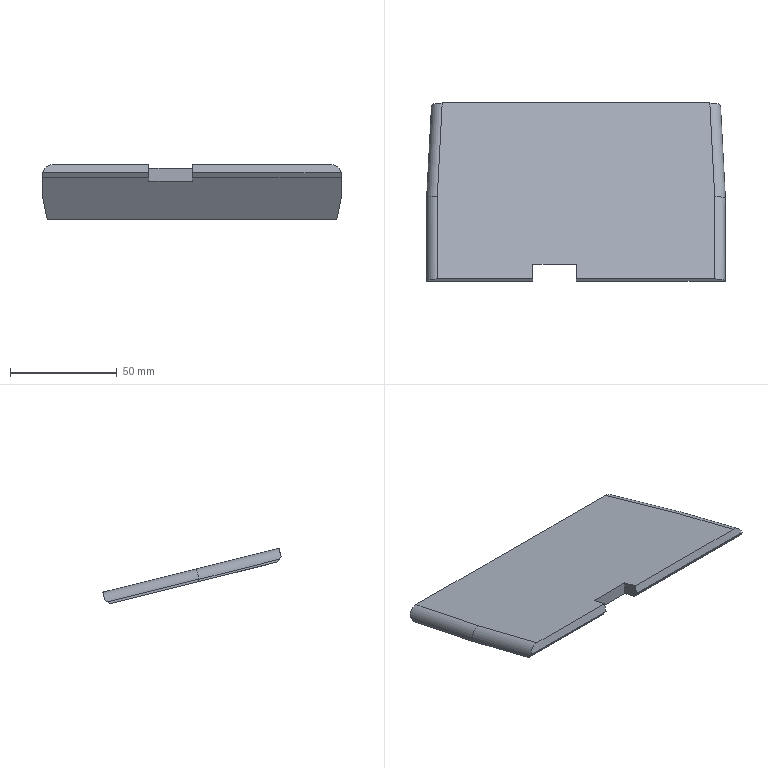Part | STEP file | WEAR-PLATE2_id674_x_t | 1 solid | 19 faces | box 140 x 83.443 x 25.901 mm | volume 68382 mm3 | plane 15 | cylinder 4 | commonest cylinder face diameters 10 x4
STEP:
#1=CARTESIAN_POINT('',(45.,1.133,224.747));
#2=VERTEX_POINT('',#1);
#3=CARTESIAN_POINT('',(50.,0.06233,219.926));
#4=VERTEX_POINT('',#3);
#5=CARTESIAN_POINT('',(45.,-0.07625,219.896));
#6=DIRECTION('',(-0.0254,0.97,-0.2418));
#7=DIRECTION('',(-0.9997,-0.02465,0.006145));
#8=AXIS2_PLACEMENT_3D('',#5,#6,#7);
#9=ELLIPSE('',#8,5.002,5.);
#10=EDGE_CURVE('',#2,#4,#9,.T.);
#11=ORIENTED_EDGE('',*,*,#10,.F.);
#12=CARTESIAN_POINT('',(45.,-37.475,234.373));
#13=VERTEX_POINT('',#12);
#14=CARTESIAN_POINT('',(45.,-37.475,234.373));
#15=DIRECTION('',(0.,0.9703,-0.2419));
#16=VECTOR('',#15,1.);
#17=LINE('',#14,#16);
#18=EDGE_CURVE('',#13,#2,#17,.T.);
#19=ORIENTED_EDGE('',*,*,#18,.F.);
#20=CARTESIAN_POINT('',(49.899,-38.443,230.492));
#21=VERTEX_POINT('',#20);
#22=CARTESIAN_POINT('',(45.,-38.685,229.522));
#23=DIRECTION('',(0.,-0.9703,0.2419));
#24=DIRECTION('',(0.,-0.2419,-0.9703));
#25=AXIS2_PLACEMENT_3D('',#22,#23,#24);
#26=CIRCLE('',#25,5.);
#27=EDGE_CURVE('',#21,#13,#26,.T.);
#28=ORIENTED_EDGE('',*,*,#27,.F.);
#29=CARTESIAN_POINT('',(50.,-37.714,229.28));
#30=VERTEX_POINT('',#29);
#31=CARTESIAN_POINT('',(45.,-37.714,229.28));
#32=DIRECTION('',(0.,0.8572,0.515));
#33=DIRECTION('',(0.,-0.515,0.8572));
#34=AXIS2_PLACEMENT_3D('',#31,#32,#33);
#35=ELLIPSE('',#34,7.071,5.);
#36=EDGE_CURVE('',#21,#30,#35,.T.);
#37=ORIENTED_EDGE('',*,*,#36,.T.);
#38=CARTESIAN_POINT('',(50.,0.05468,219.863));
#39=VERTEX_POINT('',#38);
#40=CARTESIAN_POINT('',(50.,-37.714,229.28));
#41=DIRECTION('',(0.,0.9703,-0.2419));
#42=VECTOR('',#41,1.);
#43=LINE('',#40,#42);
#44=EDGE_CURVE('',#30,#39,#43,.T.);
#45=ORIENTED_EDGE('',*,*,#44,.T.);
#46=CARTESIAN_POINT('',(50.,0.05468,219.863));
#47=CARTESIAN_POINT('',(50.,0.05468,219.885));
#48=CARTESIAN_POINT('',(50.,0.05723,219.906));
#49=CARTESIAN_POINT('',(50.,0.06233,219.926));
#50=B_SPLINE_CURVE_WITH_KNOTS('',3,(#46,#47,#48,#49),.UNSPECIFIED.,.F.,.F.,(4,4),(0.,1.),.UNSPECIFIED.);
#51=EDGE_CURVE('',#39,#4,#50,.T.);
#52=ORIENTED_EDGE('',*,*,#51,.T.);
#53=EDGE_LOOP('',(#11,#19,#28,#37,#45,#52));
#54=FACE_OUTER_BOUND('',#53,.T.);
#55=CARTESIAN_POINT('',(45.,44.241,208.846));
#56=DIRECTION('',(0.,-0.9703,0.2419));
#57=DIRECTION('',(0.,-0.2419,-0.9703));
#58=AXIS2_PLACEMENT_3D('',#55,#56,#57);
#59=CYLINDRICAL_SURFACE('',#58,5.);
#60=ADVANCED_FACE('',(#54),#59,.T.);
#61=CARTESIAN_POINT('',(-19.8,-38.443,230.492));
#62=VERTEX_POINT('',#61);
#63=CARTESIAN_POINT('',(50.,-38.443,230.492));
#64=DIRECTION('',(-1.,0.,0.));
#65=VECTOR('',#64,1.);
#66=LINE('',#63,#65);
#67=EDGE_CURVE('',#21,#62,#66,.T.);
#68=ORIENTED_EDGE('',*,*,#67,.F.);
#69=ORIENTED_EDGE('',*,*,#27,.T.);
#70=CARTESIAN_POINT('',(-19.8,-37.475,234.373));
#71=VERTEX_POINT('',#70);
#72=CARTESIAN_POINT('',(50.,-37.475,234.373));
#73=DIRECTION('',(1.,0.,0.));
#74=VECTOR('',#73,1.);
#75=LINE('',#72,#74);
#76=EDGE_CURVE('',#71,#13,#75,.T.);
#77=ORIENTED_EDGE('',*,*,#76,.F.);
#78=CARTESIAN_POINT('',(-19.8,-37.475,234.373));
#79=DIRECTION('',(0.,-0.2419,-0.9703));
#80=VECTOR('',#79,1.);
#81=LINE('',#78,#80);
#82=EDGE_CURVE('',#71,#62,#81,.T.);
#83=ORIENTED_EDGE('',*,*,#82,.T.);
#84=EDGE_LOOP('',(#68,#69,#77,#83));
#85=FACE_OUTER_BOUND('',#84,.T.);
#86=CARTESIAN_POINT('',(50.,-38.443,230.492));
#87=DIRECTION('',(0.,-0.9703,0.2419));
#88=DIRECTION('',(0.,-0.2419,-0.9703));
#89=AXIS2_PLACEMENT_3D('',#86,#87,#88);
#90=PLANE('',#89);
#91=ADVANCED_FACE('',(#85),#90,.T.);
#92=CARTESIAN_POINT('',(-85.,1.133,224.747));
#93=VERTEX_POINT('',#92);
#94=CARTESIAN_POINT('',(-82.701,45.,213.81));
#95=VERTEX_POINT('',#94);
#96=CARTESIAN_POINT('',(-82.685,45.314,213.732));
#97=DIRECTION('',(0.05079,0.969,-0.2416));
#98=VECTOR('',#97,1.);
#99=LINE('',#96,#98);
#100=EDGE_CURVE('',#93,#95,#99,.T.);
#101=ORIENTED_EDGE('',*,*,#100,.F.);
#102=CARTESIAN_POINT('',(-85.,-37.475,234.373));
#103=VERTEX_POINT('',#102);
#104=CARTESIAN_POINT('',(-85.,-37.796,234.453));
#105=DIRECTION('',(0.,0.9703,-0.2419));
#106=VECTOR('',#105,1.);
#107=LINE('',#104,#106);
#108=EDGE_CURVE('',#103,#93,#107,.T.);
#109=ORIENTED_EDGE('',*,*,#108,.F.);
#110=CARTESIAN_POINT('',(-40.2,-37.475,234.373));
#111=VERTEX_POINT('',#110);
#112=CARTESIAN_POINT('',(50.,-37.475,234.373));
#113=DIRECTION('',(-1.,0.,0.));
#114=VECTOR('',#113,1.);
#115=LINE('',#112,#114);
#116=EDGE_CURVE('',#111,#103,#115,.T.);
#117=ORIENTED_EDGE('',*,*,#116,.F.);
#118=CARTESIAN_POINT('',(-40.2,-30.5,232.634));
#119=VERTEX_POINT('',#118);
#120=CARTESIAN_POINT('',(-40.2,-37.475,234.373));
#121=DIRECTION('',(0.,0.9703,-0.2419));
#122=VECTOR('',#121,1.);
#123=LINE('',#120,#122);
#124=EDGE_CURVE('',#111,#119,#123,.T.);
#125=ORIENTED_EDGE('',*,*,#124,.T.);
#126=CARTESIAN_POINT('',(-19.8,-30.5,232.634));
#127=VERTEX_POINT('',#126);
#128=CARTESIAN_POINT('',(-19.8,-30.5,232.634));
#129=DIRECTION('',(1.,0.,0.));
#130=VECTOR('',#129,1.);
#131=LINE('',#128,#130);
#132=EDGE_CURVE('',#119,#127,#131,.T.);
#133=ORIENTED_EDGE('',*,*,#132,.T.);
#134=CARTESIAN_POINT('',(-19.8,-30.5,232.634));
#135=DIRECTION('',(0.,-0.9703,0.2419));
#136=VECTOR('',#135,1.);
#137=LINE('',#134,#136);
#138=EDGE_CURVE('',#127,#71,#137,.T.);
#139=ORIENTED_EDGE('',*,*,#138,.T.);
#140=ORIENTED_EDGE('',*,*,#76,.T.);
#141=ORIENTED_EDGE('',*,*,#18,.T.);
#142=CARTESIAN_POINT('',(42.701,45.,213.81));
#143=VERTEX_POINT('',#142);
#144=CARTESIAN_POINT('',(47.042,-37.821,234.46));
#145=DIRECTION('',(0.05079,-0.969,0.2416));
#146=VECTOR('',#145,1.);
#147=LINE('',#144,#146);
#148=EDGE_CURVE('',#143,#2,#147,.T.);
#149=ORIENTED_EDGE('',*,*,#148,.F.);
#150=CARTESIAN_POINT('',(50.,45.,213.81));
#151=DIRECTION('',(1.,0.,0.));
#152=VECTOR('',#151,1.);
#153=LINE('',#150,#152);
#154=EDGE_CURVE('',#95,#143,#153,.T.);
#155=ORIENTED_EDGE('',*,*,#154,.F.);
#156=EDGE_LOOP('',(#101,#109,#117,#125,#133,#139,#140,#141,#149,#155));
#157=FACE_OUTER_BOUND('',#156,.T.);
#158=CARTESIAN_POINT('',(50.,-37.475,234.373));
#159=DIRECTION('',(0.,0.2419,0.9703));
#160=DIRECTION('',(0.,-0.9703,0.2419));
#161=AXIS2_PLACEMENT_3D('',#158,#159,#160);
#162=PLANE('',#161);
#163=ADVANCED_FACE('',(#157),#162,.T.);
#164=ORIENTED_EDGE('',*,*,#116,.T.);
#165=CARTESIAN_POINT('',(-89.899,-38.443,230.492));
#166=VERTEX_POINT('',#165);
#167=CARTESIAN_POINT('',(-85.,-38.685,229.522));
#168=DIRECTION('',(0.,0.9703,-0.2419));
#169=DIRECTION('',(0.,0.2419,0.9703));
#170=AXIS2_PLACEMENT_3D('',#167,#168,#169);
#171=CIRCLE('',#170,5.);
#172=EDGE_CURVE('',#166,#103,#171,.T.);
#173=ORIENTED_EDGE('',*,*,#172,.F.);
#174=CARTESIAN_POINT('',(-40.2,-38.443,230.492));
#175=VERTEX_POINT('',#174);
#176=CARTESIAN_POINT('',(50.,-38.443,230.492));
#177=DIRECTION('',(-1.,0.,0.));
#178=VECTOR('',#177,1.);
#179=LINE('',#176,#178);
#180=EDGE_CURVE('',#175,#166,#179,.T.);
#181=ORIENTED_EDGE('',*,*,#180,.F.);
#182=CARTESIAN_POINT('',(-40.2,-38.443,230.492));
#183=DIRECTION('',(0.,0.2419,0.9703));
#184=VECTOR('',#183,1.);
#185=LINE('',#182,#184);
#186=EDGE_CURVE('',#175,#111,#185,.T.);
#187=ORIENTED_EDGE('',*,*,#186,.T.);
#188=EDGE_LOOP('',(#164,#173,#181,#187));
#189=FACE_OUTER_BOUND('',#188,.T.);
#190=CARTESIAN_POINT('',(50.,-38.443,230.492));
#191=DIRECTION('',(0.,-0.9703,0.2419));
#192=DIRECTION('',(0.,-0.2419,-0.9703));
#193=AXIS2_PLACEMENT_3D('',#190,#191,#192);
#194=PLANE('',#193);
#195=ADVANCED_FACE('',(#189),#194,.T.);
#196=CARTESIAN_POINT('',(-90.,0.06233,219.926));
#197=VERTEX_POINT('',#196);
#198=CARTESIAN_POINT('',(-90.,0.05468,219.863));
#199=VERTEX_POINT('',#198);
#200=CARTESIAN_POINT('',(-90.,0.06233,219.926));
#201=CARTESIAN_POINT('',(-90.,0.05723,219.906));
#202=CARTESIAN_POINT('',(-90.,0.05468,219.885));
#203=CARTESIAN_POINT('',(-90.,0.05468,219.863));
#204=B_SPLINE_CURVE_WITH_KNOTS('',3,(#200,#201,#202,#203),.UNSPECIFIED.,.F.,.F.,(4,4),(0.,1.),.UNSPECIFIED.);
#205=EDGE_CURVE('',#197,#199,#204,.T.);
#206=ORIENTED_EDGE('',*,*,#205,.T.);
#207=CARTESIAN_POINT('',(-90.,-37.714,229.28));
#208=VERTEX_POINT('',#207);
#209=CARTESIAN_POINT('',(-90.,-37.714,229.28));
#210=DIRECTION('',(0.,0.9703,-0.2419));
#211=VECTOR('',#210,1.);
#212=LINE('',#209,#211);
#213=EDGE_CURVE('',#208,#199,#212,.T.);
#214=ORIENTED_EDGE('',*,*,#213,.F.);
#215=CARTESIAN_POINT('',(-85.,-37.714,229.28));
#216=DIRECTION('',(0.,-0.8572,-0.515));
#217=DIRECTION('',(0.,0.515,-0.8572));
#218=AXIS2_PLACEMENT_3D('',#215,#216,#217);
#219=ELLIPSE('',#218,7.071,5.);
#220=EDGE_CURVE('',#166,#208,#219,.T.);
#221=ORIENTED_EDGE('',*,*,#220,.F.);
#222=ORIENTED_EDGE('',*,*,#172,.T.);
#223=ORIENTED_EDGE('',*,*,#108,.T.);
#224=CARTESIAN_POINT('',(-85.,-0.07625,219.896));
#225=DIRECTION('',(0.0254,0.97,-0.2418));
#226=DIRECTION('',(-0.9997,0.02465,-0.006145));
#227=AXIS2_PLACEMENT_3D('',#224,#225,#226);
#228=ELLIPSE('',#227,5.002,5.);
#229=EDGE_CURVE('',#197,#93,#228,.T.);
#230=ORIENTED_EDGE('',*,*,#229,.F.);
#231=EDGE_LOOP('',(#206,#214,#221,#222,#223,#230));
#232=FACE_OUTER_BOUND('',#231,.T.);
#233=CARTESIAN_POINT('',(-85.,-39.005,229.602));
#234=DIRECTION('',(0.,0.9703,-0.2419));
#235=DIRECTION('',(0.,0.2419,0.9703));
#236=AXIS2_PLACEMENT_3D('',#233,#234,#235);
#237=CYLINDRICAL_SURFACE('',#236,5.);
#238=ADVANCED_FACE('',(#232),#237,.T.);
#239=ORIENTED_EDGE('',*,*,#229,.T.);
#240=ORIENTED_EDGE('',*,*,#100,.T.);
#241=CARTESIAN_POINT('',(-87.606,44.032,209.929));
#242=VERTEX_POINT('',#241);
#243=CARTESIAN_POINT('',(-82.701,43.79,208.959));
#244=DIRECTION('',(0.,0.9703,-0.2419));
#245=DIRECTION('',(-1.,0.,0.));
#246=AXIS2_PLACEMENT_3D('',#243,#244,#245);
#247=ELLIPSE('',#246,5.006,5.);
#248=EDGE_CURVE('',#242,#95,#247,.T.);
#249=ORIENTED_EDGE('',*,*,#248,.F.);
#250=CARTESIAN_POINT('',(-87.755,42.897,209.247));
#251=VERTEX_POINT('',#250);
#252=CARTESIAN_POINT('',(-82.752,42.82,209.2));
#253=DIRECTION('',(0.,-0.515,0.8572));
#254=DIRECTION('',(-0.07173,-0.855,-0.5137));
#255=AXIS2_PLACEMENT_3D('',#252,#253,#254);
#256=ELLIPSE('',#255,7.08,5.);
#257=EDGE_CURVE('',#242,#251,#256,.T.);
#258=ORIENTED_EDGE('',*,*,#257,.T.);
#259=CARTESIAN_POINT('',(-87.755,42.897,209.247));
#260=DIRECTION('',(-0.05079,-0.969,0.2416));
#261=VECTOR('',#260,1.);
#262=LINE('',#259,#261);
#263=EDGE_CURVE('',#251,#197,#262,.T.);
#264=ORIENTED_EDGE('',*,*,#263,.T.);
#265=EDGE_LOOP('',(#239,#240,#249,#258,#264));
#266=FACE_OUTER_BOUND('',#265,.T.);
#267=CARTESIAN_POINT('',(-82.685,44.104,208.88));
#268=DIRECTION('',(-0.05079,-0.969,0.2416));
#269=DIRECTION('',(0.,-0.2419,-0.9703));
#270=AXIS2_PLACEMENT_3D('',#267,#268,#269);
#271=CYLINDRICAL_SURFACE('',#270,5.);
#272=ADVANCED_FACE('',(#266),#271,.T.);
#273=CARTESIAN_POINT('',(47.606,44.032,209.929));
#274=VERTEX_POINT('',#273);
#275=CARTESIAN_POINT('',(50.,44.032,209.929));
#276=DIRECTION('',(1.,0.,0.));
#277=VECTOR('',#276,1.);
#278=LINE('',#275,#277);
#279=EDGE_CURVE('',#242,#274,#278,.T.);
#280=ORIENTED_EDGE('',*,*,#279,.F.);
#281=ORIENTED_EDGE('',*,*,#248,.T.);
#282=ORIENTED_EDGE('',*,*,#154,.T.);
#283=CARTESIAN_POINT('',(42.701,43.79,208.959));
#284=DIRECTION('',(0.,-0.9703,0.2419));
#285=DIRECTION('',(-1.,0.,0.));
#286=AXIS2_PLACEMENT_3D('',#283,#284,#285);
#287=ELLIPSE('',#286,5.006,5.);
#288=EDGE_CURVE('',#274,#143,#287,.T.);
#289=ORIENTED_EDGE('',*,*,#288,.F.);
#290=EDGE_LOOP('',(#280,#281,#282,#289));
#291=FACE_OUTER_BOUND('',#290,.T.);
#292=CARTESIAN_POINT('',(50.,45.,213.81));
#293=DIRECTION('',(0.,0.9703,-0.2419));
#294=DIRECTION('',(0.,0.2419,0.9703));
#295=AXIS2_PLACEMENT_3D('',#292,#293,#294);
#296=PLANE('',#295);
#297=ADVANCED_FACE('',(#291),#296,.T.);
#298=ORIENTED_EDGE('',*,*,#10,.T.);
#299=CARTESIAN_POINT('',(47.755,42.897,209.247));
#300=VERTEX_POINT('',#299);
#301=CARTESIAN_POINT('',(50.,0.06233,219.926));
#302=DIRECTION('',(-0.05079,0.969,-0.2416));
#303=VECTOR('',#302,1.);
#304=LINE('',#301,#303);
#305=EDGE_CURVE('',#4,#300,#304,.T.);
#306=ORIENTED_EDGE('',*,*,#305,.T.);
#307=CARTESIAN_POINT('',(42.752,42.82,209.2));
#308=DIRECTION('',(0.,0.515,-0.8572));
#309=DIRECTION('',(-0.07173,0.855,0.5137));
#310=AXIS2_PLACEMENT_3D('',#307,#308,#309);
#311=ELLIPSE('',#310,7.08,5.);
#312=EDGE_CURVE('',#274,#300,#311,.T.);
#313=ORIENTED_EDGE('',*,*,#312,.F.);
#314=ORIENTED_EDGE('',*,*,#288,.T.);
#315=ORIENTED_EDGE('',*,*,#148,.T.);
#316=EDGE_LOOP('',(#298,#306,#313,#314,#315));
#317=FACE_OUTER_BOUND('',#316,.T.);
#318=CARTESIAN_POINT('',(47.042,-39.031,229.608));
#319=DIRECTION('',(-0.05079,0.969,-0.2416));
#320=DIRECTION('',(0.,0.2419,0.9703));
#321=AXIS2_PLACEMENT_3D('',#318,#319,#320);
#322=CYLINDRICAL_SURFACE('',#321,5.);
#323=ADVANCED_FACE('',(#317),#322,.T.);
#324=CARTESIAN_POINT('',(50.,0.05468,218.832));
#325=VERTEX_POINT('',#324);
#326=CARTESIAN_POINT('',(50.,-36.986,228.068));
#327=VERTEX_POINT('',#326);
#328=CARTESIAN_POINT('',(50.,41.608,208.472));
#329=DIRECTION('',(0.,-0.9703,0.2419));
#330=VECTOR('',#329,1.);
#331=LINE('',#328,#330);
#332=EDGE_CURVE('',#325,#327,#331,.T.);
#333=ORIENTED_EDGE('',*,*,#332,.F.);
#334=CARTESIAN_POINT('',(50.,0.05468,235.003));
#335=DIRECTION('',(0.,0.,1.));
#336=VECTOR('',#335,1.);
#337=LINE('',#334,#336);
#338=EDGE_CURVE('',#325,#39,#337,.T.);
#339=ORIENTED_EDGE('',*,*,#338,.T.);
#340=ORIENTED_EDGE('',*,*,#44,.F.);
#341=CARTESIAN_POINT('',(50.,-36.986,228.068));
#342=DIRECTION('',(0.,-0.515,0.8572));
#343=VECTOR('',#342,1.);
#344=LINE('',#341,#343);
#345=EDGE_CURVE('',#327,#30,#344,.T.);
#346=ORIENTED_EDGE('',*,*,#345,.F.);
#347=EDGE_LOOP('',(#333,#339,#340,#346));
#348=FACE_OUTER_BOUND('',#347,.T.);
#349=CARTESIAN_POINT('',(50.,60.,160.003));
#350=DIRECTION('',(-1.,0.,0.));
#351=DIRECTION('',(0.,0.,1.));
#352=AXIS2_PLACEMENT_3D('',#349,#350,#351);
#353=PLANE('',#352);
#354=ADVANCED_FACE('',(#348),#353,.F.);
#355=ORIENTED_EDGE('',*,*,#345,.T.);
#356=ORIENTED_EDGE('',*,*,#36,.F.);
#357=ORIENTED_EDGE('',*,*,#67,.T.);
#358=CARTESIAN_POINT('',(-19.8,-36.986,228.068));
#359=VERTEX_POINT('',#358);
#360=CARTESIAN_POINT('',(-19.8,-38.443,230.492));
#361=DIRECTION('',(0.,0.515,-0.8572));
#362=VECTOR('',#361,1.);
#363=LINE('',#360,#362);
#364=EDGE_CURVE('',#62,#359,#363,.T.);
#365=ORIENTED_EDGE('',*,*,#364,.T.);
#366=CARTESIAN_POINT('',(50.,-36.986,228.068));
#367=DIRECTION('',(-1.,0.,0.));
#368=VECTOR('',#367,1.);
#369=LINE('',#366,#368);
#370=EDGE_CURVE('',#327,#359,#369,.T.);
#371=ORIENTED_EDGE('',*,*,#370,.F.);
#372=EDGE_LOOP('',(#355,#356,#357,#365,#371));
#373=FACE_OUTER_BOUND('',#372,.T.);
#374=CARTESIAN_POINT('',(50.,-36.986,228.068));
#375=DIRECTION('',(0.,-0.8572,-0.515));
#376=DIRECTION('',(0.,0.515,-0.8572));
#377=AXIS2_PLACEMENT_3D('',#374,#375,#376);
#378=PLANE('',#377);
#379=ADVANCED_FACE('',(#373),#378,.T.);
#380=CARTESIAN_POINT('',(-19.8,-30.5,226.451));
#381=VERTEX_POINT('',#380);
#382=CARTESIAN_POINT('',(-19.8,-30.5,235.003));
#383=DIRECTION('',(0.,0.,-1.));
#384=VECTOR('',#383,1.);
#385=LINE('',#382,#384);
#386=EDGE_CURVE('',#127,#381,#385,.T.);
#387=ORIENTED_EDGE('',*,*,#386,.T.);
#388=CARTESIAN_POINT('',(-19.8,41.608,208.472));
#389=DIRECTION('',(0.,0.9703,-0.2419));
#390=VECTOR('',#389,1.);
#391=LINE('',#388,#390);
#392=EDGE_CURVE('',#359,#381,#391,.T.);
#393=ORIENTED_EDGE('',*,*,#392,.F.);
#394=ORIENTED_EDGE('',*,*,#364,.F.);
#395=ORIENTED_EDGE('',*,*,#82,.F.);
#396=ORIENTED_EDGE('',*,*,#138,.F.);
#397=EDGE_LOOP('',(#387,#393,#394,#395,#396));
#398=FACE_OUTER_BOUND('',#397,.T.);
#399=CARTESIAN_POINT('',(-19.8,-60.,235.003));
#400=DIRECTION('',(1.,0.,0.));
#401=DIRECTION('',(0.,0.,-1.));
#402=AXIS2_PLACEMENT_3D('',#399,#400,#401);
#403=PLANE('',#402);
#404=ADVANCED_FACE('',(#398),#403,.F.);
#405=CARTESIAN_POINT('',(-40.2,-30.5,226.451));
#406=VERTEX_POINT('',#405);
#407=CARTESIAN_POINT('',(50.,-30.5,226.451));
#408=DIRECTION('',(-1.,0.,0.));
#409=VECTOR('',#408,1.);
#410=LINE('',#407,#409);
#411=EDGE_CURVE('',#381,#406,#410,.T.);
#412=ORIENTED_EDGE('',*,*,#411,.F.);
#413=ORIENTED_EDGE('',*,*,#386,.F.);
#414=ORIENTED_EDGE('',*,*,#132,.F.);
#415=CARTESIAN_POINT('',(-40.2,-30.5,235.003));
#416=DIRECTION('',(0.,0.,-1.));
#417=VECTOR('',#416,1.);
#418=LINE('',#415,#417);
#419=EDGE_CURVE('',#119,#406,#418,.T.);
#420=ORIENTED_EDGE('',*,*,#419,.T.);
#421=EDGE_LOOP('',(#412,#413,#414,#420));
#422=FACE_OUTER_BOUND('',#421,.T.);
#423=CARTESIAN_POINT('',(-19.8,-30.5,235.003));
#424=DIRECTION('',(0.,1.,0.));
#425=DIRECTION('',(0.,0.,1.));
#426=AXIS2_PLACEMENT_3D('',#423,#424,#425);
#427=PLANE('',#426);
#428=ADVANCED_FACE('',(#422),#427,.F.);
#429=CARTESIAN_POINT('',(-40.2,-36.986,228.068));
#430=VERTEX_POINT('',#429);
#431=CARTESIAN_POINT('',(-40.2,41.608,208.472));
#432=DIRECTION('',(0.,-0.9703,0.2419));
#433=VECTOR('',#432,1.);
#434=LINE('',#431,#433);
#435=EDGE_CURVE('',#406,#430,#434,.T.);
#436=ORIENTED_EDGE('',*,*,#435,.F.);
#437=ORIENTED_EDGE('',*,*,#419,.F.);
#438=ORIENTED_EDGE('',*,*,#124,.F.);
#439=ORIENTED_EDGE('',*,*,#186,.F.);
#440=CARTESIAN_POINT('',(-40.2,-36.986,228.068));
#441=DIRECTION('',(0.,-0.515,0.8572));
#442=VECTOR('',#441,1.);
#443=LINE('',#440,#442);
#444=EDGE_CURVE('',#430,#175,#443,.T.);
#445=ORIENTED_EDGE('',*,*,#444,.F.);
#446=EDGE_LOOP('',(#436,#437,#438,#439,#445));
#447=FACE_OUTER_BOUND('',#446,.T.);
#448=CARTESIAN_POINT('',(-40.2,-30.5,235.003));
#449=DIRECTION('',(-1.,0.,0.));
#450=DIRECTION('',(0.,0.,1.));
#451=AXIS2_PLACEMENT_3D('',#448,#449,#450);
#452=PLANE('',#451);
#453=ADVANCED_FACE('',(#447),#452,.F.);
#454=ORIENTED_EDGE('',*,*,#180,.T.);
#455=ORIENTED_EDGE('',*,*,#220,.T.);
#456=CARTESIAN_POINT('',(-90.,-36.986,228.068));
#457=VERTEX_POINT('',#456);
#458=CARTESIAN_POINT('',(-90.,-36.986,228.068));
#459=DIRECTION('',(0.,-0.515,0.8572));
#460=VECTOR('',#459,1.);
#461=LINE('',#458,#460);
#462=EDGE_CURVE('',#457,#208,#461,.T.);
#463=ORIENTED_EDGE('',*,*,#462,.F.);
#464=CARTESIAN_POINT('',(50.,-36.986,228.068));
#465=DIRECTION('',(-1.,0.,0.));
#466=VECTOR('',#465,1.);
#467=LINE('',#464,#466);
#468=EDGE_CURVE('',#430,#457,#467,.T.);
#469=ORIENTED_EDGE('',*,*,#468,.F.);
#470=ORIENTED_EDGE('',*,*,#444,.T.);
#471=EDGE_LOOP('',(#454,#455,#463,#469,#470));
#472=FACE_OUTER_BOUND('',#471,.T.);
#473=CARTESIAN_POINT('',(50.,-36.986,228.068));
#474=DIRECTION('',(0.,-0.8572,-0.515));
#475=DIRECTION('',(0.,0.515,-0.8572));
#476=AXIS2_PLACEMENT_3D('',#473,#474,#475);
#477=PLANE('',#476);
#478=ADVANCED_FACE('',(#472),#477,.T.);
#479=ORIENTED_EDGE('',*,*,#462,.T.);
#480=ORIENTED_EDGE('',*,*,#213,.T.);
#481=CARTESIAN_POINT('',(-90.,0.05468,218.832));
#482=VERTEX_POINT('',#481);
#483=CARTESIAN_POINT('',(-90.,0.05468,235.003));
#484=DIRECTION('',(0.,0.,-1.));
#485=VECTOR('',#484,1.);
#486=LINE('',#483,#485);
#487=EDGE_CURVE('',#199,#482,#486,.T.);
#488=ORIENTED_EDGE('',*,*,#487,.T.);
#489=CARTESIAN_POINT('',(-90.,41.608,208.472));
#490=DIRECTION('',(0.,0.9703,-0.2419));
#491=VECTOR('',#490,1.);
#492=LINE('',#489,#491);
#493=EDGE_CURVE('',#457,#482,#492,.T.);
#494=ORIENTED_EDGE('',*,*,#493,.F.);
#495=EDGE_LOOP('',(#479,#480,#488,#494));
#496=FACE_OUTER_BOUND('',#495,.T.);
#497=CARTESIAN_POINT('',(-90.,60.,160.003));
#498=DIRECTION('',(-1.,0.,0.));
#499=DIRECTION('',(0.,0.,1.));
#500=AXIS2_PLACEMENT_3D('',#497,#498,#499);
#501=PLANE('',#500);
#502=ADVANCED_FACE('',(#496),#501,.T.);
#503=CARTESIAN_POINT('',(-87.822,41.608,208.472));
#504=VERTEX_POINT('',#503);
#505=CARTESIAN_POINT('',(-87.822,41.608,208.472));
#506=DIRECTION('',(0.04488,0.8563,0.5145));
#507=VECTOR('',#506,1.);
#508=LINE('',#505,#507);
#509=EDGE_CURVE('',#504,#251,#508,.T.);
#510=ORIENTED_EDGE('',*,*,#509,.F.);
#511=CARTESIAN_POINT('',(-90.,0.05468,218.832));
#512=DIRECTION('',(0.05079,0.969,-0.2416));
#513=VECTOR('',#512,1.);
#514=LINE('',#511,#513);
#515=EDGE_CURVE('',#482,#504,#514,.T.);
#516=ORIENTED_EDGE('',*,*,#515,.F.);
#517=ORIENTED_EDGE('',*,*,#487,.F.);
#518=ORIENTED_EDGE('',*,*,#205,.F.);
#519=ORIENTED_EDGE('',*,*,#263,.F.);
#520=EDGE_LOOP('',(#510,#516,#517,#518,#519));
#521=FACE_OUTER_BOUND('',#520,.T.);
#522=CARTESIAN_POINT('',(-90.,0.05468,235.003));
#523=DIRECTION('',(0.9986,-0.05234,0.));
#524=DIRECTION('',(0.05234,0.9986,0.));
#525=AXIS2_PLACEMENT_3D('',#522,#523,#524);
#526=PLANE('',#525);
#527=ADVANCED_FACE('',(#521),#526,.F.);
#528=ORIENTED_EDGE('',*,*,#509,.T.);
#529=ORIENTED_EDGE('',*,*,#257,.F.);
#530=ORIENTED_EDGE('',*,*,#279,.T.);
#531=ORIENTED_EDGE('',*,*,#312,.T.);
#532=CARTESIAN_POINT('',(47.822,41.608,208.472));
#533=VERTEX_POINT('',#532);
#534=CARTESIAN_POINT('',(47.755,42.897,209.247));
#535=DIRECTION('',(0.04488,-0.8563,-0.5145));
#536=VECTOR('',#535,1.);
#537=LINE('',#534,#536);
#538=EDGE_CURVE('',#300,#533,#537,.T.);
#539=ORIENTED_EDGE('',*,*,#538,.T.);
#540=CARTESIAN_POINT('',(50.,41.608,208.472));
#541=DIRECTION('',(1.,0.,0.));
#542=VECTOR('',#541,1.);
#543=LINE('',#540,#542);
#544=EDGE_CURVE('',#504,#533,#543,.T.);
#545=ORIENTED_EDGE('',*,*,#544,.F.);
#546=EDGE_LOOP('',(#528,#529,#530,#531,#539,#545));
#547=FACE_OUTER_BOUND('',#546,.T.);
#548=CARTESIAN_POINT('',(50.,44.032,209.929));
#549=DIRECTION('',(0.,0.515,-0.8572));
#550=DIRECTION('',(0.,0.8572,0.515));
#551=AXIS2_PLACEMENT_3D('',#548,#549,#550);
#552=PLANE('',#551);
#553=ADVANCED_FACE('',(#547),#552,.T.);
#554=CARTESIAN_POINT('',(47.822,41.608,208.472));
#555=DIRECTION('',(0.05079,-0.969,0.2416));
#556=VECTOR('',#555,1.);
#557=LINE('',#554,#556);
#558=EDGE_CURVE('',#533,#325,#557,.T.);
#559=ORIENTED_EDGE('',*,*,#558,.F.);
#560=ORIENTED_EDGE('',*,*,#538,.F.);
#561=ORIENTED_EDGE('',*,*,#305,.F.);
#562=ORIENTED_EDGE('',*,*,#51,.F.);
#563=ORIENTED_EDGE('',*,*,#338,.F.);
#564=EDGE_LOOP('',(#559,#560,#561,#562,#563));
#565=FACE_OUTER_BOUND('',#564,.T.);
#566=CARTESIAN_POINT('',(47.645,45.,235.003));
#567=DIRECTION('',(-0.9986,-0.05234,0.));
#568=DIRECTION('',(0.05234,-0.9986,0.));
#569=AXIS2_PLACEMENT_3D('',#566,#567,#568);
#570=PLANE('',#569);
#571=ADVANCED_FACE('',(#565),#570,.F.);
#572=ORIENTED_EDGE('',*,*,#544,.T.);
#573=ORIENTED_EDGE('',*,*,#558,.T.);
#574=ORIENTED_EDGE('',*,*,#332,.T.);
#575=ORIENTED_EDGE('',*,*,#370,.T.);
#576=ORIENTED_EDGE('',*,*,#392,.T.);
#577=ORIENTED_EDGE('',*,*,#411,.T.);
#578=ORIENTED_EDGE('',*,*,#435,.T.);
#579=ORIENTED_EDGE('',*,*,#468,.T.);
#580=ORIENTED_EDGE('',*,*,#493,.T.);
#581=ORIENTED_EDGE('',*,*,#515,.T.);
#582=EDGE_LOOP('',(#572,#573,#574,#575,#576,#577,#578,#579,#580,#581));
#583=FACE_OUTER_BOUND('',#582,.T.);
#584=CARTESIAN_POINT('',(50.,41.608,208.472));
#585=DIRECTION('',(0.,-0.2419,-0.9703));
#586=DIRECTION('',(0.,0.9703,-0.2419));
#587=AXIS2_PLACEMENT_3D('',#584,#585,#586);
#588=PLANE('',#587);
#589=ADVANCED_FACE('',(#583),#588,.T.);
#590=CLOSED_SHELL('',(#60,#91,#163,#195,#238,#272,#297,#323,#354,#379,#404,#428,#453,#478,#502,#527,#553,#571,#589));
#591=MANIFOLD_SOLID_BREP('',#590);
#592=(LENGTH_UNIT()NAMED_UNIT(*)SI_UNIT(.MILLI.,.METRE.));
#593=UNCERTAINTY_MEASURE_WITH_UNIT(LENGTH_MEASURE(0.0508),#592,'','');
#594=(NAMED_UNIT(*)PLANE_ANGLE_UNIT()SI_UNIT($,.RADIAN.));
#595=PLANE_ANGLE_MEASURE_WITH_UNIT(PLANE_ANGLE_MEASURE(0.01745),#594);
#596=DIMENSIONAL_EXPONENTS(0.,0.,0.,0.,0.,0.,0.);
#597=(CONVERSION_BASED_UNIT('DEGREE',#595)NAMED_UNIT(#596)PLANE_ANGLE_UNIT());
#598=(NAMED_UNIT(*)SI_UNIT($,.STERADIAN.)SOLID_ANGLE_UNIT());
#599=(GEOMETRIC_REPRESENTATION_CONTEXT(3)GLOBAL_UNCERTAINTY_ASSIGNED_CONTEXT((#593))GLOBAL_UNIT_ASSIGNED_CONTEXT((#592,#597,#598))REPRESENTATION_CONTEXT('',''));
#600=ADVANCED_BREP_SHAPE_REPRESENTATION('',(#591),#599);